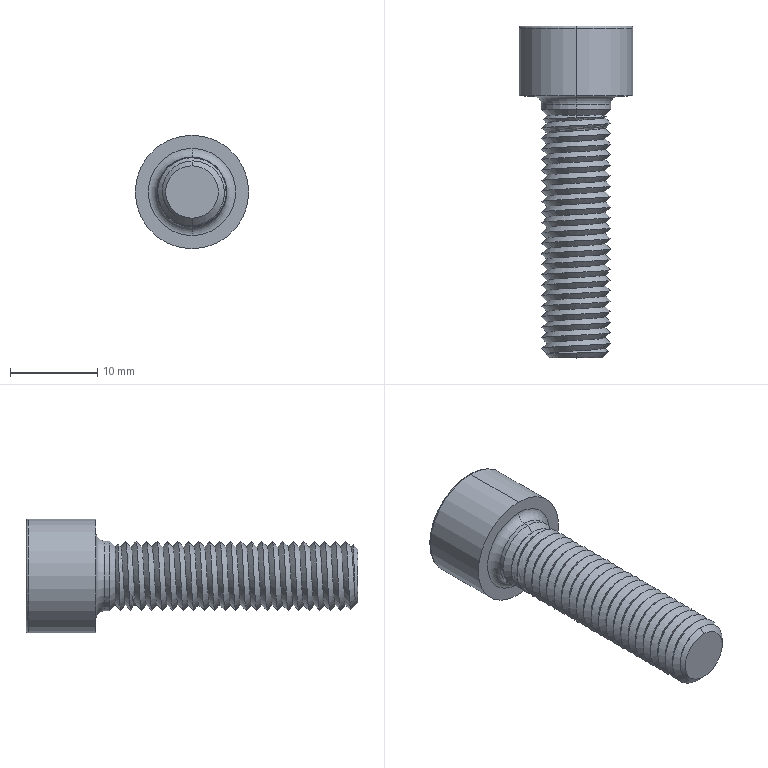Part | STEP file | Parafuso M8 - 30mm | 1 solid | 36 faces | box 13 x 38 x 13 mm | volume 2114 mm3 | plane 16 | cone 8 | torus 6 | cylinder 4 | spline 2 | commonest cylinder face diameters 8 x2 13 x2